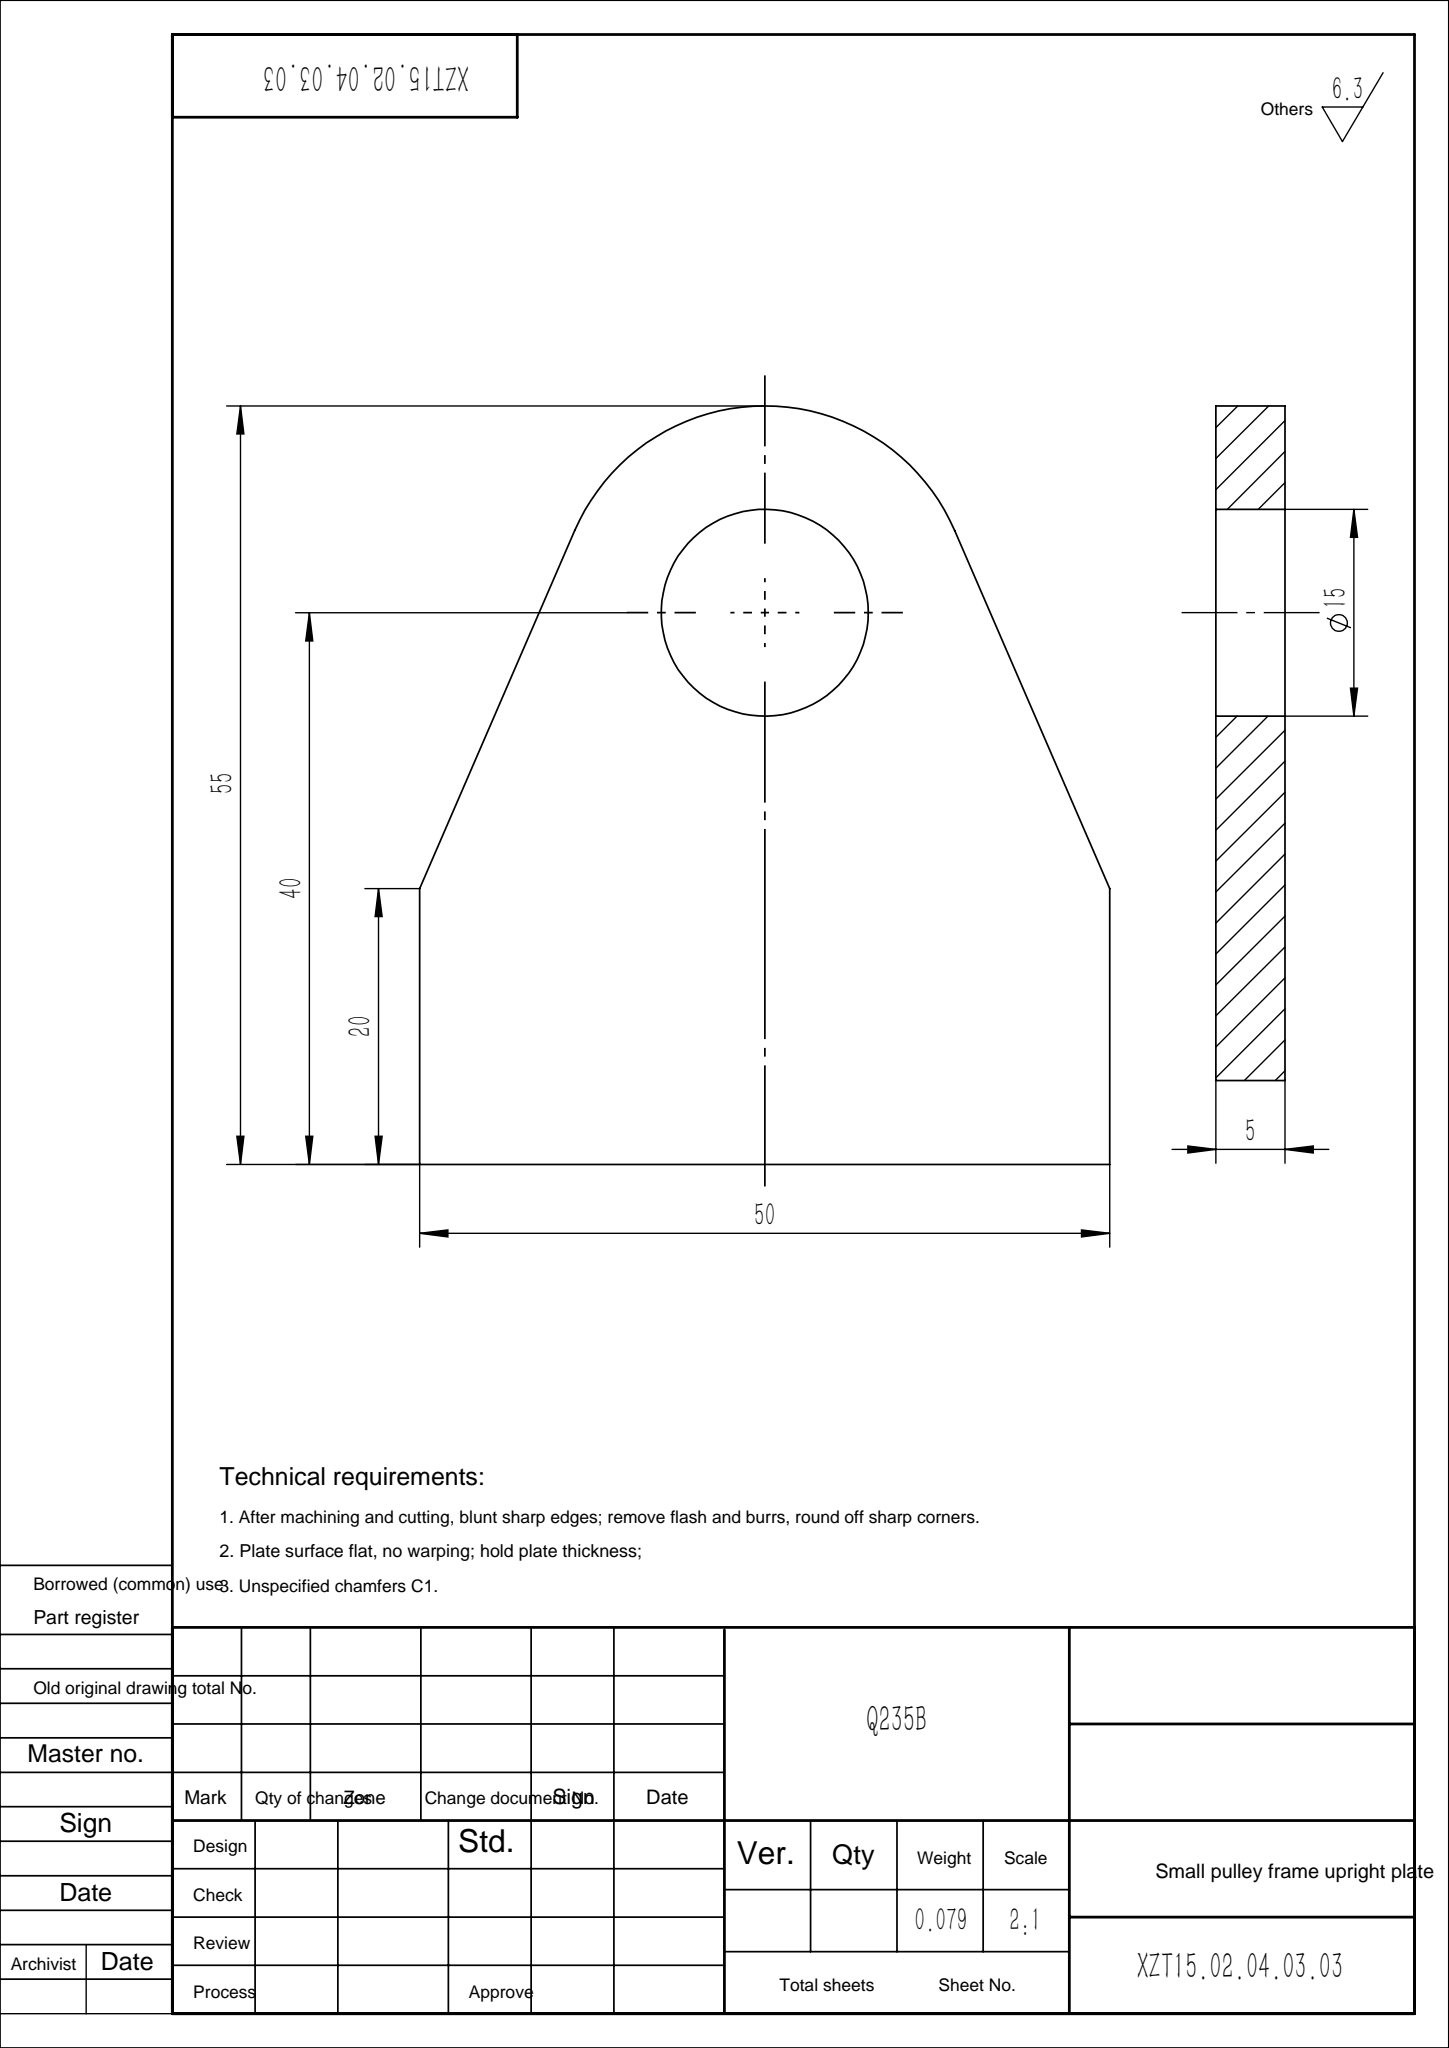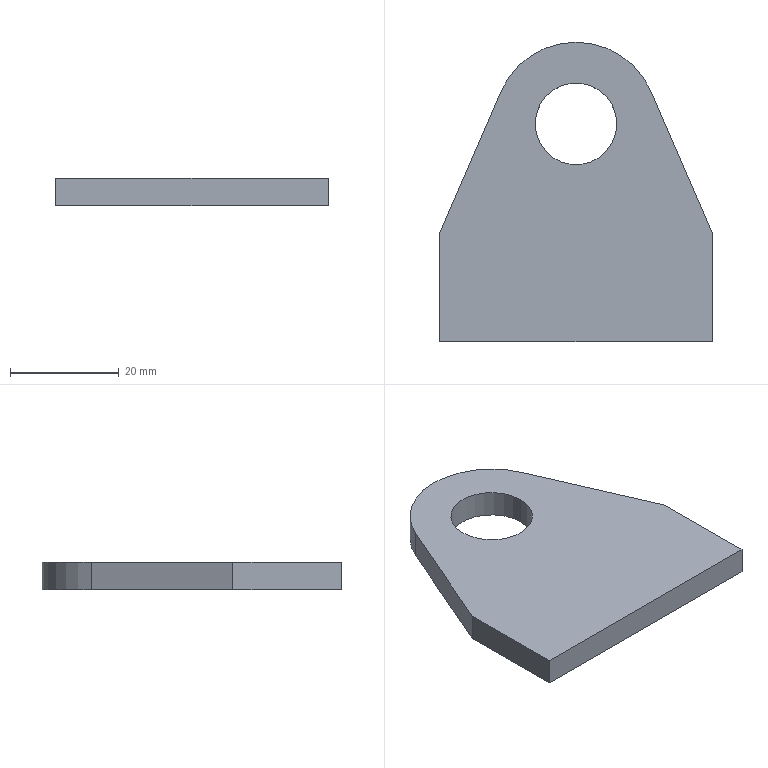Part | SolidWorks | features Extrusion 1, ICE 1 | 1 solid | 10 faces | box 50 x 55 x 5 mm | volume 10045 mm3 | plane 7 | cylinder 3 | commonest cylinder face diameters 15 x2 30 x1
STEP:
#1=CARTESIAN_POINT('',(-7.5,20.,2.5));
#2=VERTEX_POINT('',#1);
#3=CARTESIAN_POINT('',(7.5,20.,2.5));
#4=VERTEX_POINT('',#3);
#5=CARTESIAN_POINT('',(0.,20.,2.5));
#6=DIRECTION('',(0.,0.,1.));
#7=DIRECTION('',(1.,0.,0.));
#8=AXIS2_PLACEMENT_3D('',#5,#6,#7);
#9=CIRCLE('',#8,7.5);
#10=EDGE_CURVE('',#2,#4,#9,.T.);
#11=ORIENTED_EDGE('',*,*,#10,.T.);
#12=CARTESIAN_POINT('',(7.5,20.,-2.5));
#13=VERTEX_POINT('',#12);
#14=CARTESIAN_POINT('',(7.5,20.,2.5));
#15=DIRECTION('',(0.,0.,-1.));
#16=VECTOR('',#15,1000.);
#17=LINE('',#14,#16);
#18=EDGE_CURVE('',#4,#13,#17,.T.);
#19=ORIENTED_EDGE('',*,*,#18,.T.);
#20=CARTESIAN_POINT('',(-7.5,20.,-2.5));
#21=VERTEX_POINT('',#20);
#22=CARTESIAN_POINT('',(0.,20.,-2.5));
#23=DIRECTION('',(0.,0.,1.));
#24=DIRECTION('',(1.,0.,0.));
#25=AXIS2_PLACEMENT_3D('',#22,#23,#24);
#26=CIRCLE('',#25,7.5);
#27=EDGE_CURVE('',#21,#13,#26,.T.);
#28=ORIENTED_EDGE('',*,*,#27,.F.);
#29=CARTESIAN_POINT('',(-7.5,20.,2.5));
#30=DIRECTION('',(0.,0.,-1.));
#31=VECTOR('',#30,1000.);
#32=LINE('',#29,#31);
#33=EDGE_CURVE('',#2,#21,#32,.T.);
#34=ORIENTED_EDGE('',*,*,#33,.F.);
#35=EDGE_LOOP('',(#11,#19,#28,#34));
#36=FACE_OUTER_BOUND('',#35,.T.);
#37=CARTESIAN_POINT('',(0.,20.,2.5));
#38=DIRECTION('',(0.,0.,-1.));
#39=DIRECTION('',(-1.,0.,0.));
#40=AXIS2_PLACEMENT_3D('',#37,#38,#39);
#41=CYLINDRICAL_SURFACE('',#40,7.5);
#42=ADVANCED_FACE('',(#36),#41,.F.);
#43=CARTESIAN_POINT('',(-13.766,25.958,2.5));
#44=VERTEX_POINT('',#43);
#45=CARTESIAN_POINT('',(-25.,0.,2.5));
#46=VERTEX_POINT('',#45);
#47=CARTESIAN_POINT('',(-25.,0.,2.5));
#48=DIRECTION('',(-0.3972,-0.9177,0.));
#49=VECTOR('',#48,1000.);
#50=LINE('',#47,#49);
#51=EDGE_CURVE('',#44,#46,#50,.T.);
#52=ORIENTED_EDGE('',*,*,#51,.T.);
#53=CARTESIAN_POINT('',(-25.,-20.,2.5));
#54=VERTEX_POINT('',#53);
#55=CARTESIAN_POINT('',(-25.,0.,2.5));
#56=DIRECTION('',(0.,-1.,0.));
#57=VECTOR('',#56,1000.);
#58=LINE('',#55,#57);
#59=EDGE_CURVE('',#46,#54,#58,.T.);
#60=ORIENTED_EDGE('',*,*,#59,.T.);
#61=CARTESIAN_POINT('',(25.,-20.,2.5));
#62=VERTEX_POINT('',#61);
#63=CARTESIAN_POINT('',(-25.,-20.,2.5));
#64=DIRECTION('',(1.,0.,0.));
#65=VECTOR('',#64,1000.);
#66=LINE('',#63,#65);
#67=EDGE_CURVE('',#54,#62,#66,.T.);
#68=ORIENTED_EDGE('',*,*,#67,.T.);
#69=CARTESIAN_POINT('',(25.,0.,2.5));
#70=VERTEX_POINT('',#69);
#71=CARTESIAN_POINT('',(25.,0.,2.5));
#72=DIRECTION('',(0.,1.,0.));
#73=VECTOR('',#72,1000.);
#74=LINE('',#71,#73);
#75=EDGE_CURVE('',#62,#70,#74,.T.);
#76=ORIENTED_EDGE('',*,*,#75,.T.);
#77=CARTESIAN_POINT('',(13.766,25.958,2.5));
#78=VERTEX_POINT('',#77);
#79=CARTESIAN_POINT('',(25.,0.,2.5));
#80=DIRECTION('',(-0.3972,0.9177,0.));
#81=VECTOR('',#80,1000.);
#82=LINE('',#79,#81);
#83=EDGE_CURVE('',#70,#78,#82,.T.);
#84=ORIENTED_EDGE('',*,*,#83,.T.);
#85=CARTESIAN_POINT('',(0.,20.,2.5));
#86=DIRECTION('',(0.,0.,1.));
#87=DIRECTION('',(-1.,0.,0.));
#88=AXIS2_PLACEMENT_3D('',#85,#86,#87);
#89=CIRCLE('',#88,15.);
#90=EDGE_CURVE('',#78,#44,#89,.T.);
#91=ORIENTED_EDGE('',*,*,#90,.T.);
#92=EDGE_LOOP('',(#52,#60,#68,#76,#84,#91));
#93=FACE_OUTER_BOUND('',#92,.T.);
#94=ORIENTED_EDGE('',*,*,#10,.F.);
#95=CARTESIAN_POINT('',(0.,20.,2.5));
#96=DIRECTION('',(0.,0.,1.));
#97=DIRECTION('',(1.,0.,0.));
#98=AXIS2_PLACEMENT_3D('',#95,#96,#97);
#99=CIRCLE('',#98,7.5);
#100=EDGE_CURVE('',#4,#2,#99,.T.);
#101=ORIENTED_EDGE('',*,*,#100,.F.);
#102=EDGE_LOOP('',(#94,#101));
#103=FACE_BOUND('',#102,.T.);
#104=CARTESIAN_POINT('',(0.,20.,2.5));
#105=DIRECTION('',(0.,0.,-1.));
#106=DIRECTION('',(-1.,0.,0.));
#107=AXIS2_PLACEMENT_3D('',#104,#105,#106);
#108=PLANE('',#107);
#109=ADVANCED_FACE('',(#93,#103),#108,.F.);
#110=CARTESIAN_POINT('',(-13.766,25.958,-2.5));
#111=VERTEX_POINT('',#110);
#112=CARTESIAN_POINT('',(-25.,0.,-2.5));
#113=VERTEX_POINT('',#112);
#114=CARTESIAN_POINT('',(-25.,0.,-2.5));
#115=DIRECTION('',(-0.3972,-0.9177,0.));
#116=VECTOR('',#115,1000.);
#117=LINE('',#114,#116);
#118=EDGE_CURVE('',#111,#113,#117,.T.);
#119=ORIENTED_EDGE('',*,*,#118,.F.);
#120=CARTESIAN_POINT('',(13.766,25.958,-2.5));
#121=VERTEX_POINT('',#120);
#122=CARTESIAN_POINT('',(0.,20.,-2.5));
#123=DIRECTION('',(0.,0.,1.));
#124=DIRECTION('',(-1.,0.,0.));
#125=AXIS2_PLACEMENT_3D('',#122,#123,#124);
#126=CIRCLE('',#125,15.);
#127=EDGE_CURVE('',#121,#111,#126,.T.);
#128=ORIENTED_EDGE('',*,*,#127,.F.);
#129=CARTESIAN_POINT('',(25.,0.,-2.5));
#130=VERTEX_POINT('',#129);
#131=CARTESIAN_POINT('',(25.,0.,-2.5));
#132=DIRECTION('',(-0.3972,0.9177,0.));
#133=VECTOR('',#132,1000.);
#134=LINE('',#131,#133);
#135=EDGE_CURVE('',#130,#121,#134,.T.);
#136=ORIENTED_EDGE('',*,*,#135,.F.);
#137=CARTESIAN_POINT('',(25.,-20.,-2.5));
#138=VERTEX_POINT('',#137);
#139=CARTESIAN_POINT('',(25.,0.,-2.5));
#140=DIRECTION('',(0.,1.,0.));
#141=VECTOR('',#140,1000.);
#142=LINE('',#139,#141);
#143=EDGE_CURVE('',#138,#130,#142,.T.);
#144=ORIENTED_EDGE('',*,*,#143,.F.);
#145=CARTESIAN_POINT('',(-25.,-20.,-2.5));
#146=VERTEX_POINT('',#145);
#147=CARTESIAN_POINT('',(-25.,-20.,-2.5));
#148=DIRECTION('',(1.,0.,0.));
#149=VECTOR('',#148,1000.);
#150=LINE('',#147,#149);
#151=EDGE_CURVE('',#146,#138,#150,.T.);
#152=ORIENTED_EDGE('',*,*,#151,.F.);
#153=CARTESIAN_POINT('',(-25.,0.,-2.5));
#154=DIRECTION('',(0.,-1.,0.));
#155=VECTOR('',#154,1000.);
#156=LINE('',#153,#155);
#157=EDGE_CURVE('',#113,#146,#156,.T.);
#158=ORIENTED_EDGE('',*,*,#157,.F.);
#159=EDGE_LOOP('',(#119,#128,#136,#144,#152,#158));
#160=FACE_OUTER_BOUND('',#159,.T.);
#161=ORIENTED_EDGE('',*,*,#27,.T.);
#162=CARTESIAN_POINT('',(0.,20.,-2.5));
#163=DIRECTION('',(0.,0.,1.));
#164=DIRECTION('',(1.,0.,0.));
#165=AXIS2_PLACEMENT_3D('',#162,#163,#164);
#166=CIRCLE('',#165,7.5);
#167=EDGE_CURVE('',#13,#21,#166,.T.);
#168=ORIENTED_EDGE('',*,*,#167,.T.);
#169=EDGE_LOOP('',(#161,#168));
#170=FACE_BOUND('',#169,.T.);
#171=CARTESIAN_POINT('',(0.,20.,-2.5));
#172=DIRECTION('',(0.,0.,-1.));
#173=DIRECTION('',(-1.,0.,0.));
#174=AXIS2_PLACEMENT_3D('',#171,#172,#173);
#175=PLANE('',#174);
#176=ADVANCED_FACE('',(#160,#170),#175,.T.);
#177=ORIENTED_EDGE('',*,*,#118,.T.);
#178=CARTESIAN_POINT('',(-25.,0.,2.5));
#179=DIRECTION('',(0.,0.,-1.));
#180=VECTOR('',#179,1000.);
#181=LINE('',#178,#180);
#182=EDGE_CURVE('',#46,#113,#181,.T.);
#183=ORIENTED_EDGE('',*,*,#182,.F.);
#184=ORIENTED_EDGE('',*,*,#51,.F.);
#185=CARTESIAN_POINT('',(-13.766,25.958,2.5));
#186=DIRECTION('',(0.,0.,-1.));
#187=VECTOR('',#186,1000.);
#188=LINE('',#185,#187);
#189=EDGE_CURVE('',#44,#111,#188,.T.);
#190=ORIENTED_EDGE('',*,*,#189,.T.);
#191=EDGE_LOOP('',(#177,#183,#184,#190));
#192=FACE_OUTER_BOUND('',#191,.T.);
#193=CARTESIAN_POINT('',(-25.,0.,2.5));
#194=DIRECTION('',(0.9177,-0.3972,0.));
#195=DIRECTION('',(0.3972,0.9177,0.));
#196=AXIS2_PLACEMENT_3D('',#193,#194,#195);
#197=PLANE('',#196);
#198=ADVANCED_FACE('',(#192),#197,.F.);
#199=ORIENTED_EDGE('',*,*,#135,.T.);
#200=CARTESIAN_POINT('',(13.766,25.958,2.5));
#201=DIRECTION('',(0.,0.,-1.));
#202=VECTOR('',#201,1000.);
#203=LINE('',#200,#202);
#204=EDGE_CURVE('',#78,#121,#203,.T.);
#205=ORIENTED_EDGE('',*,*,#204,.F.);
#206=ORIENTED_EDGE('',*,*,#83,.F.);
#207=CARTESIAN_POINT('',(25.,0.,2.5));
#208=DIRECTION('',(0.,0.,-1.));
#209=VECTOR('',#208,1000.);
#210=LINE('',#207,#209);
#211=EDGE_CURVE('',#70,#130,#210,.T.);
#212=ORIENTED_EDGE('',*,*,#211,.T.);
#213=EDGE_LOOP('',(#199,#205,#206,#212));
#214=FACE_OUTER_BOUND('',#213,.T.);
#215=CARTESIAN_POINT('',(25.,0.,2.5));
#216=DIRECTION('',(-0.9177,-0.3972,0.));
#217=DIRECTION('',(0.3972,-0.9177,0.));
#218=AXIS2_PLACEMENT_3D('',#215,#216,#217);
#219=PLANE('',#218);
#220=ADVANCED_FACE('',(#214),#219,.F.);
#221=ORIENTED_EDGE('',*,*,#127,.T.);
#222=ORIENTED_EDGE('',*,*,#189,.F.);
#223=ORIENTED_EDGE('',*,*,#90,.F.);
#224=ORIENTED_EDGE('',*,*,#204,.T.);
#225=EDGE_LOOP('',(#221,#222,#223,#224));
#226=FACE_OUTER_BOUND('',#225,.T.);
#227=CARTESIAN_POINT('',(0.,20.,2.5));
#228=DIRECTION('',(0.,0.,-1.));
#229=DIRECTION('',(-1.,0.,0.));
#230=AXIS2_PLACEMENT_3D('',#227,#228,#229);
#231=CYLINDRICAL_SURFACE('',#230,15.);
#232=ADVANCED_FACE('',(#226),#231,.T.);
#233=ORIENTED_EDGE('',*,*,#18,.F.);
#234=ORIENTED_EDGE('',*,*,#100,.T.);
#235=ORIENTED_EDGE('',*,*,#33,.T.);
#236=ORIENTED_EDGE('',*,*,#167,.F.);
#237=EDGE_LOOP('',(#233,#234,#235,#236));
#238=FACE_OUTER_BOUND('',#237,.T.);
#239=CARTESIAN_POINT('',(0.,20.,2.5));
#240=DIRECTION('',(0.,0.,-1.));
#241=DIRECTION('',(-1.,0.,0.));
#242=AXIS2_PLACEMENT_3D('',#239,#240,#241);
#243=CYLINDRICAL_SURFACE('',#242,7.5);
#244=ADVANCED_FACE('',(#238),#243,.F.);
#245=ORIENTED_EDGE('',*,*,#59,.F.);
#246=ORIENTED_EDGE('',*,*,#182,.T.);
#247=ORIENTED_EDGE('',*,*,#157,.T.);
#248=CARTESIAN_POINT('',(-25.,-20.,-2.5));
#249=DIRECTION('',(0.,0.,1.));
#250=VECTOR('',#249,1000.);
#251=LINE('',#248,#250);
#252=EDGE_CURVE('',#146,#54,#251,.T.);
#253=ORIENTED_EDGE('',*,*,#252,.T.);
#254=EDGE_LOOP('',(#245,#246,#247,#253));
#255=FACE_OUTER_BOUND('',#254,.T.);
#256=CARTESIAN_POINT('',(-25.,0.,-2.5));
#257=DIRECTION('',(-1.,0.,0.));
#258=DIRECTION('',(0.,-1.,0.));
#259=AXIS2_PLACEMENT_3D('',#256,#257,#258);
#260=PLANE('',#259);
#261=ADVANCED_FACE('',(#255),#260,.T.);
#262=ORIENTED_EDGE('',*,*,#75,.F.);
#263=CARTESIAN_POINT('',(25.,-20.,-2.5));
#264=DIRECTION('',(0.,0.,1.));
#265=VECTOR('',#264,1000.);
#266=LINE('',#263,#265);
#267=EDGE_CURVE('',#138,#62,#266,.T.);
#268=ORIENTED_EDGE('',*,*,#267,.F.);
#269=ORIENTED_EDGE('',*,*,#143,.T.);
#270=ORIENTED_EDGE('',*,*,#211,.F.);
#271=EDGE_LOOP('',(#262,#268,#269,#270));
#272=FACE_OUTER_BOUND('',#271,.T.);
#273=CARTESIAN_POINT('',(25.,0.,-2.5));
#274=DIRECTION('',(1.,0.,0.));
#275=DIRECTION('',(0.,0.,-1.));
#276=AXIS2_PLACEMENT_3D('',#273,#274,#275);
#277=PLANE('',#276);
#278=ADVANCED_FACE('',(#272),#277,.T.);
#279=ORIENTED_EDGE('',*,*,#67,.F.);
#280=ORIENTED_EDGE('',*,*,#252,.F.);
#281=ORIENTED_EDGE('',*,*,#151,.T.);
#282=ORIENTED_EDGE('',*,*,#267,.T.);
#283=EDGE_LOOP('',(#279,#280,#281,#282));
#284=FACE_OUTER_BOUND('',#283,.T.);
#285=CARTESIAN_POINT('',(-25.,-20.,-2.5));
#286=DIRECTION('',(0.,-1.,0.));
#287=DIRECTION('',(0.,0.,-1.));
#288=AXIS2_PLACEMENT_3D('',#285,#286,#287);
#289=PLANE('',#288);
#290=ADVANCED_FACE('',(#284),#289,.T.);
#291=CLOSED_SHELL('',(#42,#109,#176,#198,#220,#232,#244,#261,#278,#290));
#292=MANIFOLD_SOLID_BREP('',#291);
#293=CARTESIAN_POINT('',(0.,0.,0.));
#294=DIRECTION('',(0.,0.,1.));
#295=DIRECTION('',(1.,0.,0.));
#296=AXIS2_PLACEMENT_3D('',#293,#294,#295);
#297=(LENGTH_UNIT()NAMED_UNIT(*)SI_UNIT(.MILLI.,.METRE.));
#298=UNCERTAINTY_MEASURE_WITH_UNIT(LENGTH_MEASURE(0.00001),#297,'','');
#299=(NAMED_UNIT(*)PLANE_ANGLE_UNIT()SI_UNIT($,.RADIAN.));
#300=(NAMED_UNIT(*)SI_UNIT($,.STERADIAN.)SOLID_ANGLE_UNIT());
#301=(GEOMETRIC_REPRESENTATION_CONTEXT(3)GLOBAL_UNCERTAINTY_ASSIGNED_CONTEXT((#298))GLOBAL_UNIT_ASSIGNED_CONTEXT((#297,#299,#300))REPRESENTATION_CONTEXT('',''));
#302=ADVANCED_BREP_SHAPE_REPRESENTATION('',(#292,#296),#301);